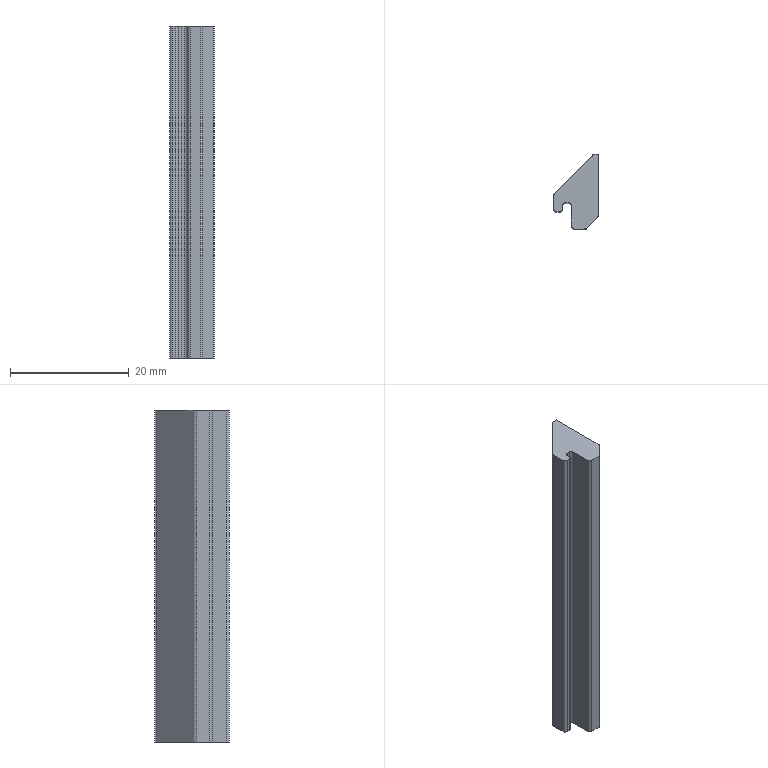Part | NX | features BREP 2 | 2 solids | 42 faces | box 7.556 x 12.583 x 56 mm | volume 6581 mm3 | plane 24 | cylinder 18 | commonest cylinder face diameters 1 x18
STEP:
#1=CARTESIAN_POINT('',(3.778,-3.929,-4.));
#2=VERTEX_POINT('',#1);
#3=CARTESIAN_POINT('',(3.778,-3.929,52.));
#4=VERTEX_POINT('',#3);
#5=CARTESIAN_POINT('',(3.778,-3.929,0.));
#6=DIRECTION('',(0.,0.,1.));
#7=VECTOR('',#6,1000.);
#8=LINE('',#5,#7);
#9=EDGE_CURVE('',#2,#4,#8,.T.);
#10=ORIENTED_EDGE('',*,*,#9,.T.);
#11=CARTESIAN_POINT('',(3.632,-4.282,52.));
#12=VERTEX_POINT('',#11);
#13=CARTESIAN_POINT('',(3.278,-3.929,52.));
#14=DIRECTION('',(0.,0.,1.));
#15=DIRECTION('',(1.,0.,0.));
#16=AXIS2_PLACEMENT_3D('',#13,#14,#15);
#17=CIRCLE('',#16,0.5);
#18=EDGE_CURVE('',#12,#4,#17,.T.);
#19=ORIENTED_EDGE('',*,*,#18,.F.);
#20=CARTESIAN_POINT('',(3.632,-4.282,-4.));
#21=VERTEX_POINT('',#20);
#22=CARTESIAN_POINT('',(3.632,-4.282,0.));
#23=DIRECTION('',(0.,0.,1.));
#24=VECTOR('',#23,1000.);
#25=LINE('',#22,#24);
#26=EDGE_CURVE('',#21,#12,#25,.T.);
#27=ORIENTED_EDGE('',*,*,#26,.F.);
#28=CARTESIAN_POINT('',(3.278,-3.929,-4.));
#29=DIRECTION('',(0.,0.,1.));
#30=DIRECTION('',(1.,0.,0.));
#31=AXIS2_PLACEMENT_3D('',#28,#29,#30);
#32=CIRCLE('',#31,0.5);
#33=EDGE_CURVE('',#21,#2,#32,.T.);
#34=ORIENTED_EDGE('',*,*,#33,.T.);
#35=EDGE_LOOP('',(#10,#19,#27,#34));
#36=FACE_BOUND('',#35,.T.);
#37=CARTESIAN_POINT('',(3.278,-3.929,0.));
#38=DIRECTION('',(0.,0.,1.));
#39=DIRECTION('',(-1.,0.,0.));
#40=AXIS2_PLACEMENT_3D('',#37,#38,#39);
#41=CYLINDRICAL_SURFACE('',#40,0.5);
#42=ADVANCED_FACE('',(#36),#41,.T.);
#43=ORIENTED_EDGE('',*,*,#26,.T.);
#44=CARTESIAN_POINT('',(1.768,-6.145,52.));
#45=VERTEX_POINT('',#44);
#46=CARTESIAN_POINT('',(3.632,-4.282,52.));
#47=DIRECTION('',(0.7071,0.7071,0.));
#48=VECTOR('',#47,1000.);
#49=LINE('',#46,#48);
#50=EDGE_CURVE('',#45,#12,#49,.T.);
#51=ORIENTED_EDGE('',*,*,#50,.F.);
#52=CARTESIAN_POINT('',(1.768,-6.145,-4.));
#53=VERTEX_POINT('',#52);
#54=CARTESIAN_POINT('',(1.768,-6.145,0.));
#55=DIRECTION('',(0.,0.,1.));
#56=VECTOR('',#55,1000.);
#57=LINE('',#54,#56);
#58=EDGE_CURVE('',#53,#45,#57,.T.);
#59=ORIENTED_EDGE('',*,*,#58,.F.);
#60=CARTESIAN_POINT('',(3.632,-4.282,-4.));
#61=DIRECTION('',(0.7071,0.7071,0.));
#62=VECTOR('',#61,1000.);
#63=LINE('',#60,#62);
#64=EDGE_CURVE('',#53,#21,#63,.T.);
#65=ORIENTED_EDGE('',*,*,#64,.T.);
#66=EDGE_LOOP('',(#43,#51,#59,#65));
#67=FACE_BOUND('',#66,.T.);
#68=CARTESIAN_POINT('',(3.632,-4.282,0.));
#69=DIRECTION('',(-0.7071,0.7071,0.));
#70=DIRECTION('',(0.7071,0.7071,0.));
#71=AXIS2_PLACEMENT_3D('',#68,#69,#70);
#72=PLANE('',#71);
#73=ADVANCED_FACE('',(#67),#72,.F.);
#74=ORIENTED_EDGE('',*,*,#58,.T.);
#75=CARTESIAN_POINT('',(1.415,-6.292,52.));
#76=VERTEX_POINT('',#75);
#77=CARTESIAN_POINT('',(1.415,-5.792,52.));
#78=DIRECTION('',(0.,0.,1.));
#79=DIRECTION('',(1.,0.,0.));
#80=AXIS2_PLACEMENT_3D('',#77,#78,#79);
#81=CIRCLE('',#80,0.5);
#82=EDGE_CURVE('',#76,#45,#81,.T.);
#83=ORIENTED_EDGE('',*,*,#82,.F.);
#84=CARTESIAN_POINT('',(1.415,-6.292,-4.));
#85=VERTEX_POINT('',#84);
#86=CARTESIAN_POINT('',(1.415,-6.292,0.));
#87=DIRECTION('',(0.,0.,1.));
#88=VECTOR('',#87,1000.);
#89=LINE('',#86,#88);
#90=EDGE_CURVE('',#85,#76,#89,.T.);
#91=ORIENTED_EDGE('',*,*,#90,.F.);
#92=CARTESIAN_POINT('',(1.415,-5.792,-4.));
#93=DIRECTION('',(0.,0.,1.));
#94=DIRECTION('',(1.,0.,0.));
#95=AXIS2_PLACEMENT_3D('',#92,#93,#94);
#96=CIRCLE('',#95,0.5);
#97=EDGE_CURVE('',#85,#53,#96,.T.);
#98=ORIENTED_EDGE('',*,*,#97,.T.);
#99=EDGE_LOOP('',(#74,#83,#91,#98));
#100=FACE_BOUND('',#99,.T.);
#101=CARTESIAN_POINT('',(1.415,-5.792,0.));
#102=DIRECTION('',(0.,0.,1.));
#103=DIRECTION('',(-1.,0.,0.));
#104=AXIS2_PLACEMENT_3D('',#101,#102,#103);
#105=CYLINDRICAL_SURFACE('',#104,0.5);
#106=ADVANCED_FACE('',(#100),#105,.T.);
#107=ORIENTED_EDGE('',*,*,#90,.T.);
#108=CARTESIAN_POINT('',(-0.278,-6.292,52.));
#109=VERTEX_POINT('',#108);
#110=CARTESIAN_POINT('',(-3.752,-6.292,52.));
#111=DIRECTION('',(1.,0.,0.));
#112=VECTOR('',#111,1000.);
#113=LINE('',#110,#112);
#114=EDGE_CURVE('',#109,#76,#113,.T.);
#115=ORIENTED_EDGE('',*,*,#114,.F.);
#116=CARTESIAN_POINT('',(-0.278,-6.292,-4.));
#117=VERTEX_POINT('',#116);
#118=CARTESIAN_POINT('',(-0.278,-6.292,0.));
#119=DIRECTION('',(0.,0.,1.));
#120=VECTOR('',#119,1000.);
#121=LINE('',#118,#120);
#122=EDGE_CURVE('',#117,#109,#121,.T.);
#123=ORIENTED_EDGE('',*,*,#122,.F.);
#124=CARTESIAN_POINT('',(-3.752,-6.292,-4.));
#125=DIRECTION('',(1.,0.,0.));
#126=VECTOR('',#125,1000.);
#127=LINE('',#124,#126);
#128=EDGE_CURVE('',#117,#85,#127,.T.);
#129=ORIENTED_EDGE('',*,*,#128,.T.);
#130=EDGE_LOOP('',(#107,#115,#123,#129));
#131=FACE_BOUND('',#130,.T.);
#132=CARTESIAN_POINT('',(1.415,-6.292,0.));
#133=DIRECTION('',(0.,1.,0.));
#134=DIRECTION('',(1.,0.,0.));
#135=AXIS2_PLACEMENT_3D('',#132,#133,#134);
#136=PLANE('',#135);
#137=ADVANCED_FACE('',(#131),#136,.F.);
#138=ORIENTED_EDGE('',*,*,#122,.T.);
#139=CARTESIAN_POINT('',(-0.778,-5.792,52.));
#140=VERTEX_POINT('',#139);
#141=CARTESIAN_POINT('',(-0.278,-5.792,52.));
#142=DIRECTION('',(0.,0.,1.));
#143=DIRECTION('',(1.,0.,0.));
#144=AXIS2_PLACEMENT_3D('',#141,#142,#143);
#145=CIRCLE('',#144,0.5);
#146=EDGE_CURVE('',#140,#109,#145,.T.);
#147=ORIENTED_EDGE('',*,*,#146,.F.);
#148=CARTESIAN_POINT('',(-0.778,-5.792,-4.));
#149=VERTEX_POINT('',#148);
#150=CARTESIAN_POINT('',(-0.778,-5.792,0.));
#151=DIRECTION('',(0.,0.,1.));
#152=VECTOR('',#151,1000.);
#153=LINE('',#150,#152);
#154=EDGE_CURVE('',#149,#140,#153,.T.);
#155=ORIENTED_EDGE('',*,*,#154,.F.);
#156=CARTESIAN_POINT('',(-0.278,-5.792,-4.));
#157=DIRECTION('',(0.,0.,1.));
#158=DIRECTION('',(1.,0.,0.));
#159=AXIS2_PLACEMENT_3D('',#156,#157,#158);
#160=CIRCLE('',#159,0.5);
#161=EDGE_CURVE('',#149,#117,#160,.T.);
#162=ORIENTED_EDGE('',*,*,#161,.T.);
#163=EDGE_LOOP('',(#138,#147,#155,#162));
#164=FACE_BOUND('',#163,.T.);
#165=CARTESIAN_POINT('',(-0.278,-5.792,0.));
#166=DIRECTION('',(0.,0.,1.));
#167=DIRECTION('',(-1.,0.,0.));
#168=AXIS2_PLACEMENT_3D('',#165,#166,#167);
#169=CYLINDRICAL_SURFACE('',#168,0.5);
#170=ADVANCED_FACE('',(#164),#169,.T.);
#171=ORIENTED_EDGE('',*,*,#154,.T.);
#172=CARTESIAN_POINT('',(-0.778,-2.392,52.));
#173=VERTEX_POINT('',#172);
#174=CARTESIAN_POINT('',(-0.778,-5.414,52.));
#175=DIRECTION('',(0.,-1.,0.));
#176=VECTOR('',#175,1000.);
#177=LINE('',#174,#176);
#178=EDGE_CURVE('',#173,#140,#177,.T.);
#179=ORIENTED_EDGE('',*,*,#178,.F.);
#180=CARTESIAN_POINT('',(-0.778,-2.392,-4.));
#181=VERTEX_POINT('',#180);
#182=CARTESIAN_POINT('',(-0.778,-2.392,0.));
#183=DIRECTION('',(0.,0.,1.));
#184=VECTOR('',#183,1000.);
#185=LINE('',#182,#184);
#186=EDGE_CURVE('',#181,#173,#185,.T.);
#187=ORIENTED_EDGE('',*,*,#186,.F.);
#188=CARTESIAN_POINT('',(-0.778,-5.414,-4.));
#189=DIRECTION('',(0.,-1.,0.));
#190=VECTOR('',#189,1000.);
#191=LINE('',#188,#190);
#192=EDGE_CURVE('',#181,#149,#191,.T.);
#193=ORIENTED_EDGE('',*,*,#192,.T.);
#194=EDGE_LOOP('',(#171,#179,#187,#193));
#195=FACE_BOUND('',#194,.T.);
#196=CARTESIAN_POINT('',(-0.778,-5.792,0.));
#197=DIRECTION('',(1.,0.,0.));
#198=DIRECTION('',(0.,-1.,0.));
#199=AXIS2_PLACEMENT_3D('',#196,#197,#198);
#200=PLANE('',#199);
#201=ADVANCED_FACE('',(#195),#200,.F.);
#202=ORIENTED_EDGE('',*,*,#186,.T.);
#203=CARTESIAN_POINT('',(-1.278,-1.892,52.));
#204=VERTEX_POINT('',#203);
#205=CARTESIAN_POINT('',(-1.278,-2.392,52.));
#206=DIRECTION('',(0.,0.,-1.));
#207=DIRECTION('',(1.,0.,0.));
#208=AXIS2_PLACEMENT_3D('',#205,#206,#207);
#209=CIRCLE('',#208,0.5);
#210=EDGE_CURVE('',#204,#173,#209,.T.);
#211=ORIENTED_EDGE('',*,*,#210,.F.);
#212=CARTESIAN_POINT('',(-1.278,-1.892,-4.));
#213=VERTEX_POINT('',#212);
#214=CARTESIAN_POINT('',(-1.278,-1.892,0.));
#215=DIRECTION('',(0.,0.,1.));
#216=VECTOR('',#215,1000.);
#217=LINE('',#214,#216);
#218=EDGE_CURVE('',#213,#204,#217,.T.);
#219=ORIENTED_EDGE('',*,*,#218,.F.);
#220=CARTESIAN_POINT('',(-1.278,-2.392,-4.));
#221=DIRECTION('',(0.,0.,-1.));
#222=DIRECTION('',(1.,0.,0.));
#223=AXIS2_PLACEMENT_3D('',#220,#221,#222);
#224=CIRCLE('',#223,0.5);
#225=EDGE_CURVE('',#213,#181,#224,.T.);
#226=ORIENTED_EDGE('',*,*,#225,.T.);
#227=EDGE_LOOP('',(#202,#211,#219,#226));
#228=FACE_BOUND('',#227,.T.);
#229=CARTESIAN_POINT('',(-1.278,-2.392,0.));
#230=DIRECTION('',(0.,0.,1.));
#231=DIRECTION('',(-1.,0.,0.));
#232=AXIS2_PLACEMENT_3D('',#229,#230,#231);
#233=CYLINDRICAL_SURFACE('',#232,0.5);
#234=ADVANCED_FACE('',(#228),#233,.F.);
#235=ORIENTED_EDGE('',*,*,#218,.T.);
#236=CARTESIAN_POINT('',(-1.778,-1.892,52.));
#237=VERTEX_POINT('',#236);
#238=CARTESIAN_POINT('',(-3.752,-1.892,52.));
#239=DIRECTION('',(1.,0.,0.));
#240=VECTOR('',#239,1000.);
#241=LINE('',#238,#240);
#242=EDGE_CURVE('',#237,#204,#241,.T.);
#243=ORIENTED_EDGE('',*,*,#242,.F.);
#244=CARTESIAN_POINT('',(-1.778,-1.892,-4.));
#245=VERTEX_POINT('',#244);
#246=CARTESIAN_POINT('',(-1.778,-1.892,0.));
#247=DIRECTION('',(0.,0.,1.));
#248=VECTOR('',#247,1000.);
#249=LINE('',#246,#248);
#250=EDGE_CURVE('',#245,#237,#249,.T.);
#251=ORIENTED_EDGE('',*,*,#250,.F.);
#252=CARTESIAN_POINT('',(-3.752,-1.892,-4.));
#253=DIRECTION('',(1.,0.,0.));
#254=VECTOR('',#253,1000.);
#255=LINE('',#252,#254);
#256=EDGE_CURVE('',#245,#213,#255,.T.);
#257=ORIENTED_EDGE('',*,*,#256,.T.);
#258=EDGE_LOOP('',(#235,#243,#251,#257));
#259=FACE_BOUND('',#258,.T.);
#260=CARTESIAN_POINT('',(-1.278,-1.892,0.));
#261=DIRECTION('',(0.,1.,0.));
#262=DIRECTION('',(1.,0.,0.));
#263=AXIS2_PLACEMENT_3D('',#260,#261,#262);
#264=PLANE('',#263);
#265=ADVANCED_FACE('',(#259),#264,.F.);
#266=ORIENTED_EDGE('',*,*,#250,.T.);
#267=CARTESIAN_POINT('',(-2.278,-2.392,52.));
#268=VERTEX_POINT('',#267);
#269=CARTESIAN_POINT('',(-1.778,-2.392,52.));
#270=DIRECTION('',(0.,0.,-1.));
#271=DIRECTION('',(1.,0.,0.));
#272=AXIS2_PLACEMENT_3D('',#269,#270,#271);
#273=CIRCLE('',#272,0.5);
#274=EDGE_CURVE('',#268,#237,#273,.T.);
#275=ORIENTED_EDGE('',*,*,#274,.F.);
#276=CARTESIAN_POINT('',(-2.278,-2.392,-4.));
#277=VERTEX_POINT('',#276);
#278=CARTESIAN_POINT('',(-2.278,-2.392,0.));
#279=DIRECTION('',(0.,0.,1.));
#280=VECTOR('',#279,1000.);
#281=LINE('',#278,#280);
#282=EDGE_CURVE('',#277,#268,#281,.T.);
#283=ORIENTED_EDGE('',*,*,#282,.F.);
#284=CARTESIAN_POINT('',(-1.778,-2.392,-4.));
#285=DIRECTION('',(0.,0.,-1.));
#286=DIRECTION('',(1.,0.,0.));
#287=AXIS2_PLACEMENT_3D('',#284,#285,#286);
#288=CIRCLE('',#287,0.5);
#289=EDGE_CURVE('',#277,#245,#288,.T.);
#290=ORIENTED_EDGE('',*,*,#289,.T.);
#291=EDGE_LOOP('',(#266,#275,#283,#290));
#292=FACE_BOUND('',#291,.T.);
#293=CARTESIAN_POINT('',(-1.778,-2.392,0.));
#294=DIRECTION('',(0.,0.,1.));
#295=DIRECTION('',(-1.,0.,0.));
#296=AXIS2_PLACEMENT_3D('',#293,#294,#295);
#297=CYLINDRICAL_SURFACE('',#296,0.5);
#298=ADVANCED_FACE('',(#292),#297,.F.);
#299=ORIENTED_EDGE('',*,*,#282,.T.);
#300=CARTESIAN_POINT('',(-2.278,-2.892,52.));
#301=VERTEX_POINT('',#300);
#302=CARTESIAN_POINT('',(-2.278,-5.414,52.));
#303=DIRECTION('',(0.,1.,0.));
#304=VECTOR('',#303,1000.);
#305=LINE('',#302,#304);
#306=EDGE_CURVE('',#301,#268,#305,.T.);
#307=ORIENTED_EDGE('',*,*,#306,.F.);
#308=CARTESIAN_POINT('',(-2.278,-2.892,-4.));
#309=VERTEX_POINT('',#308);
#310=CARTESIAN_POINT('',(-2.278,-2.892,0.));
#311=DIRECTION('',(0.,0.,1.));
#312=VECTOR('',#311,1000.);
#313=LINE('',#310,#312);
#314=EDGE_CURVE('',#309,#301,#313,.T.);
#315=ORIENTED_EDGE('',*,*,#314,.F.);
#316=CARTESIAN_POINT('',(-2.278,-5.414,-4.));
#317=DIRECTION('',(0.,1.,0.));
#318=VECTOR('',#317,1000.);
#319=LINE('',#316,#318);
#320=EDGE_CURVE('',#309,#277,#319,.T.);
#321=ORIENTED_EDGE('',*,*,#320,.T.);
#322=EDGE_LOOP('',(#299,#307,#315,#321));
#323=FACE_BOUND('',#322,.T.);
#324=CARTESIAN_POINT('',(-2.278,-2.392,0.));
#325=DIRECTION('',(-1.,0.,0.));
#326=DIRECTION('',(0.,1.,0.));
#327=AXIS2_PLACEMENT_3D('',#324,#325,#326);
#328=PLANE('',#327);
#329=ADVANCED_FACE('',(#323),#328,.F.);
#330=ORIENTED_EDGE('',*,*,#314,.T.);
#331=CARTESIAN_POINT('',(-2.778,-3.392,52.));
#332=VERTEX_POINT('',#331);
#333=CARTESIAN_POINT('',(-2.778,-2.892,52.));
#334=DIRECTION('',(0.,0.,1.));
#335=DIRECTION('',(1.,0.,0.));
#336=AXIS2_PLACEMENT_3D('',#333,#334,#335);
#337=CIRCLE('',#336,0.5);
#338=EDGE_CURVE('',#332,#301,#337,.T.);
#339=ORIENTED_EDGE('',*,*,#338,.F.);
#340=CARTESIAN_POINT('',(-2.778,-3.392,-4.));
#341=VERTEX_POINT('',#340);
#342=CARTESIAN_POINT('',(-2.778,-3.392,0.));
#343=DIRECTION('',(0.,0.,1.));
#344=VECTOR('',#343,1000.);
#345=LINE('',#342,#344);
#346=EDGE_CURVE('',#341,#332,#345,.T.);
#347=ORIENTED_EDGE('',*,*,#346,.F.);
#348=CARTESIAN_POINT('',(-2.778,-2.892,-4.));
#349=DIRECTION('',(0.,0.,1.));
#350=DIRECTION('',(1.,0.,0.));
#351=AXIS2_PLACEMENT_3D('',#348,#349,#350);
#352=CIRCLE('',#351,0.5);
#353=EDGE_CURVE('',#341,#309,#352,.T.);
#354=ORIENTED_EDGE('',*,*,#353,.T.);
#355=EDGE_LOOP('',(#330,#339,#347,#354));
#356=FACE_BOUND('',#355,.T.);
#357=CARTESIAN_POINT('',(-2.778,-2.892,0.));
#358=DIRECTION('',(0.,0.,1.));
#359=DIRECTION('',(-1.,0.,0.));
#360=AXIS2_PLACEMENT_3D('',#357,#358,#359);
#361=CYLINDRICAL_SURFACE('',#360,0.5);
#362=ADVANCED_FACE('',(#356),#361,.T.);
#363=ORIENTED_EDGE('',*,*,#346,.T.);
#364=CARTESIAN_POINT('',(-3.278,-3.392,52.));
#365=VERTEX_POINT('',#364);
#366=CARTESIAN_POINT('',(-3.752,-3.392,52.));
#367=DIRECTION('',(1.,0.,0.));
#368=VECTOR('',#367,1000.);
#369=LINE('',#366,#368);
#370=EDGE_CURVE('',#365,#332,#369,.T.);
#371=ORIENTED_EDGE('',*,*,#370,.F.);
#372=CARTESIAN_POINT('',(-3.278,-3.392,-4.));
#373=VERTEX_POINT('',#372);
#374=CARTESIAN_POINT('',(-3.278,-3.392,0.));
#375=DIRECTION('',(0.,0.,1.));
#376=VECTOR('',#375,1000.);
#377=LINE('',#374,#376);
#378=EDGE_CURVE('',#373,#365,#377,.T.);
#379=ORIENTED_EDGE('',*,*,#378,.F.);
#380=CARTESIAN_POINT('',(-3.752,-3.392,-4.));
#381=DIRECTION('',(1.,0.,0.));
#382=VECTOR('',#381,1000.);
#383=LINE('',#380,#382);
#384=EDGE_CURVE('',#373,#341,#383,.T.);
#385=ORIENTED_EDGE('',*,*,#384,.T.);
#386=EDGE_LOOP('',(#363,#371,#379,#385));
#387=FACE_BOUND('',#386,.T.);
#388=CARTESIAN_POINT('',(-2.778,-3.392,0.));
#389=DIRECTION('',(0.,1.,0.));
#390=DIRECTION('',(1.,0.,0.));
#391=AXIS2_PLACEMENT_3D('',#388,#389,#390);
#392=PLANE('',#391);
#393=ADVANCED_FACE('',(#387),#392,.F.);
#394=ORIENTED_EDGE('',*,*,#378,.T.);
#395=CARTESIAN_POINT('',(-3.778,-2.892,52.));
#396=VERTEX_POINT('',#395);
#397=CARTESIAN_POINT('',(-3.278,-2.892,52.));
#398=DIRECTION('',(0.,0.,1.));
#399=DIRECTION('',(1.,0.,0.));
#400=AXIS2_PLACEMENT_3D('',#397,#398,#399);
#401=CIRCLE('',#400,0.5);
#402=EDGE_CURVE('',#396,#365,#401,.T.);
#403=ORIENTED_EDGE('',*,*,#402,.F.);
#404=CARTESIAN_POINT('',(-3.778,-2.892,-4.));
#405=VERTEX_POINT('',#404);
#406=CARTESIAN_POINT('',(-3.778,-2.892,0.));
#407=DIRECTION('',(0.,0.,1.));
#408=VECTOR('',#407,1000.);
#409=LINE('',#406,#408);
#410=EDGE_CURVE('',#405,#396,#409,.T.);
#411=ORIENTED_EDGE('',*,*,#410,.F.);
#412=CARTESIAN_POINT('',(-3.278,-2.892,-4.));
#413=DIRECTION('',(0.,0.,1.));
#414=DIRECTION('',(1.,0.,0.));
#415=AXIS2_PLACEMENT_3D('',#412,#413,#414);
#416=CIRCLE('',#415,0.5);
#417=EDGE_CURVE('',#405,#373,#416,.T.);
#418=ORIENTED_EDGE('',*,*,#417,.T.);
#419=EDGE_LOOP('',(#394,#403,#411,#418));
#420=FACE_BOUND('',#419,.T.);
#421=CARTESIAN_POINT('',(-3.278,-2.892,0.));
#422=DIRECTION('',(0.,0.,1.));
#423=DIRECTION('',(-1.,0.,0.));
#424=AXIS2_PLACEMENT_3D('',#421,#422,#423);
#425=CYLINDRICAL_SURFACE('',#424,0.5);
#426=ADVANCED_FACE('',(#420),#425,.T.);
#427=ORIENTED_EDGE('',*,*,#410,.T.);
#428=CARTESIAN_POINT('',(-3.778,-0.6987,52.));
#429=VERTEX_POINT('',#428);
#430=CARTESIAN_POINT('',(-3.778,-5.414,52.));
#431=DIRECTION('',(0.,-1.,0.));
#432=VECTOR('',#431,1000.);
#433=LINE('',#430,#432);
#434=EDGE_CURVE('',#429,#396,#433,.T.);
#435=ORIENTED_EDGE('',*,*,#434,.F.);
#436=CARTESIAN_POINT('',(-3.778,-0.6987,-4.));
#437=VERTEX_POINT('',#436);
#438=CARTESIAN_POINT('',(-3.778,-0.6987,0.));
#439=DIRECTION('',(0.,0.,1.));
#440=VECTOR('',#439,1000.);
#441=LINE('',#438,#440);
#442=EDGE_CURVE('',#437,#429,#441,.T.);
#443=ORIENTED_EDGE('',*,*,#442,.F.);
#444=CARTESIAN_POINT('',(-3.778,-5.414,-4.));
#445=DIRECTION('',(0.,-1.,0.));
#446=VECTOR('',#445,1000.);
#447=LINE('',#444,#446);
#448=EDGE_CURVE('',#437,#405,#447,.T.);
#449=ORIENTED_EDGE('',*,*,#448,.T.);
#450=EDGE_LOOP('',(#427,#435,#443,#449));
#451=FACE_BOUND('',#450,.T.);
#452=CARTESIAN_POINT('',(-3.778,-2.892,0.));
#453=DIRECTION('',(1.,0.,0.));
#454=DIRECTION('',(0.,-1.,0.));
#455=AXIS2_PLACEMENT_3D('',#452,#453,#454);
#456=PLANE('',#455);
#457=ADVANCED_FACE('',(#451),#456,.F.);
#458=ORIENTED_EDGE('',*,*,#442,.T.);
#459=CARTESIAN_POINT('',(-3.632,-0.3452,52.));
#460=VERTEX_POINT('',#459);
#461=CARTESIAN_POINT('',(-3.278,-0.6987,52.));
#462=DIRECTION('',(0.,0.,1.));
#463=DIRECTION('',(1.,0.,0.));
#464=AXIS2_PLACEMENT_3D('',#461,#462,#463);
#465=CIRCLE('',#464,0.5);
#466=EDGE_CURVE('',#460,#429,#465,.T.);
#467=ORIENTED_EDGE('',*,*,#466,.F.);
#468=CARTESIAN_POINT('',(-3.632,-0.3452,-4.));
#469=VERTEX_POINT('',#468);
#470=CARTESIAN_POINT('',(-3.632,-0.3452,0.));
#471=DIRECTION('',(0.,0.,1.));
#472=VECTOR('',#471,1000.);
#473=LINE('',#470,#472);
#474=EDGE_CURVE('',#469,#460,#473,.T.);
#475=ORIENTED_EDGE('',*,*,#474,.F.);
#476=CARTESIAN_POINT('',(-3.278,-0.6987,-4.));
#477=DIRECTION('',(0.,0.,1.));
#478=DIRECTION('',(1.,0.,0.));
#479=AXIS2_PLACEMENT_3D('',#476,#477,#478);
#480=CIRCLE('',#479,0.5);
#481=EDGE_CURVE('',#469,#437,#480,.T.);
#482=ORIENTED_EDGE('',*,*,#481,.T.);
#483=EDGE_LOOP('',(#458,#467,#475,#482));
#484=FACE_BOUND('',#483,.T.);
#485=CARTESIAN_POINT('',(-3.278,-0.6987,0.));
#486=DIRECTION('',(0.,0.,1.));
#487=DIRECTION('',(-1.,0.,0.));
#488=AXIS2_PLACEMENT_3D('',#485,#486,#487);
#489=CYLINDRICAL_SURFACE('',#488,0.5);
#490=ADVANCED_FACE('',(#484),#489,.T.);
#491=ORIENTED_EDGE('',*,*,#474,.T.);
#492=CARTESIAN_POINT('',(2.652,5.938,52.));
#493=VERTEX_POINT('',#492);
#494=CARTESIAN_POINT('',(-3.632,-0.3452,52.));
#495=DIRECTION('',(-0.7071,-0.7071,0.));
#496=VECTOR('',#495,1000.);
#497=LINE('',#494,#496);
#498=EDGE_CURVE('',#493,#460,#497,.T.);
#499=ORIENTED_EDGE('',*,*,#498,.F.);
#500=CARTESIAN_POINT('',(2.652,5.938,-4.));
#501=VERTEX_POINT('',#500);
#502=CARTESIAN_POINT('',(2.652,5.938,0.));
#503=DIRECTION('',(0.,0.,1.));
#504=VECTOR('',#503,1000.);
#505=LINE('',#502,#504);
#506=EDGE_CURVE('',#501,#493,#505,.T.);
#507=ORIENTED_EDGE('',*,*,#506,.F.);
#508=CARTESIAN_POINT('',(-3.632,-0.3452,-4.));
#509=DIRECTION('',(-0.7071,-0.7071,0.));
#510=VECTOR('',#509,1000.);
#511=LINE('',#508,#510);
#512=EDGE_CURVE('',#501,#469,#511,.T.);
#513=ORIENTED_EDGE('',*,*,#512,.T.);
#514=EDGE_LOOP('',(#491,#499,#507,#513));
#515=FACE_BOUND('',#514,.T.);
#516=CARTESIAN_POINT('',(-3.632,-0.3452,0.));
#517=DIRECTION('',(0.7071,-0.7071,0.));
#518=DIRECTION('',(-0.7071,-0.7071,0.));
#519=AXIS2_PLACEMENT_3D('',#516,#517,#518);
#520=PLANE('',#519);
#521=ADVANCED_FACE('',(#515),#520,.F.);
#522=ORIENTED_EDGE('',*,*,#506,.T.);
#523=CARTESIAN_POINT('',(2.798,6.292,52.));
#524=VERTEX_POINT('',#523);
#525=CARTESIAN_POINT('',(2.298,6.292,52.));
#526=DIRECTION('',(0.,0.,-1.));
#527=DIRECTION('',(1.,0.,0.));
#528=AXIS2_PLACEMENT_3D('',#525,#526,#527);
#529=CIRCLE('',#528,0.5);
#530=EDGE_CURVE('',#524,#493,#529,.T.);
#531=ORIENTED_EDGE('',*,*,#530,.F.);
#532=CARTESIAN_POINT('',(2.798,6.292,-4.));
#533=VERTEX_POINT('',#532);
#534=CARTESIAN_POINT('',(2.798,6.292,0.));
#535=DIRECTION('',(0.,0.,1.));
#536=VECTOR('',#535,1000.);
#537=LINE('',#534,#536);
#538=EDGE_CURVE('',#533,#524,#537,.T.);
#539=ORIENTED_EDGE('',*,*,#538,.F.);
#540=CARTESIAN_POINT('',(2.298,6.292,-4.));
#541=DIRECTION('',(0.,0.,-1.));
#542=DIRECTION('',(1.,0.,0.));
#543=AXIS2_PLACEMENT_3D('',#540,#541,#542);
#544=CIRCLE('',#543,0.5);
#545=EDGE_CURVE('',#533,#501,#544,.T.);
#546=ORIENTED_EDGE('',*,*,#545,.T.);
#547=EDGE_LOOP('',(#522,#531,#539,#546));
#548=FACE_BOUND('',#547,.T.);
#549=CARTESIAN_POINT('',(2.298,6.292,0.));
#550=DIRECTION('',(0.,0.,1.));
#551=DIRECTION('',(-1.,0.,0.));
#552=AXIS2_PLACEMENT_3D('',#549,#550,#551);
#553=CYLINDRICAL_SURFACE('',#552,0.5);
#554=ADVANCED_FACE('',(#548),#553,.F.);
#555=ORIENTED_EDGE('',*,*,#538,.T.);
#556=CARTESIAN_POINT('',(3.778,6.292,52.));
#557=VERTEX_POINT('',#556);
#558=CARTESIAN_POINT('',(-3.752,6.292,52.));
#559=DIRECTION('',(-1.,0.,0.));
#560=VECTOR('',#559,1000.);
#561=LINE('',#558,#560);
#562=EDGE_CURVE('',#557,#524,#561,.T.);
#563=ORIENTED_EDGE('',*,*,#562,.F.);
#564=CARTESIAN_POINT('',(3.778,6.292,-4.));
#565=VERTEX_POINT('',#564);
#566=CARTESIAN_POINT('',(3.778,6.292,0.));
#567=DIRECTION('',(0.,0.,1.));
#568=VECTOR('',#567,1000.);
#569=LINE('',#566,#568);
#570=EDGE_CURVE('',#565,#557,#569,.T.);
#571=ORIENTED_EDGE('',*,*,#570,.F.);
#572=CARTESIAN_POINT('',(-3.752,6.292,-4.));
#573=DIRECTION('',(-1.,0.,0.));
#574=VECTOR('',#573,1000.);
#575=LINE('',#572,#574);
#576=EDGE_CURVE('',#565,#533,#575,.T.);
#577=ORIENTED_EDGE('',*,*,#576,.T.);
#578=EDGE_LOOP('',(#555,#563,#571,#577));
#579=FACE_BOUND('',#578,.T.);
#580=CARTESIAN_POINT('',(-3.752,6.292,0.));
#581=DIRECTION('',(0.,-1.,0.));
#582=DIRECTION('',(-1.,0.,0.));
#583=AXIS2_PLACEMENT_3D('',#580,#581,#582);
#584=PLANE('',#583);
#585=ADVANCED_FACE('',(#579),#584,.F.);
#586=CARTESIAN_POINT('',(3.778,-5.414,-4.));
#587=DIRECTION('',(0.,1.,0.));
#588=VECTOR('',#587,1000.);
#589=LINE('',#586,#588);
#590=EDGE_CURVE('',#2,#565,#589,.T.);
#591=ORIENTED_EDGE('',*,*,#590,.T.);
#592=ORIENTED_EDGE('',*,*,#570,.T.);
#593=CARTESIAN_POINT('',(3.778,-5.414,52.));
#594=DIRECTION('',(0.,1.,0.));
#595=VECTOR('',#594,1000.);
#596=LINE('',#593,#595);
#597=EDGE_CURVE('',#4,#557,#596,.T.);
#598=ORIENTED_EDGE('',*,*,#597,.F.);
#599=ORIENTED_EDGE('',*,*,#9,.F.);
#600=EDGE_LOOP('',(#591,#592,#598,#599));
#601=FACE_BOUND('',#600,.T.);
#602=CARTESIAN_POINT('',(3.778,8.984,0.));
#603=DIRECTION('',(-1.,0.,0.));
#604=DIRECTION('',(0.,1.,0.));
#605=AXIS2_PLACEMENT_3D('',#602,#603,#604);
#606=PLANE('',#605);
#607=ADVANCED_FACE('',(#601),#606,.F.);
#608=ORIENTED_EDGE('',*,*,#562,.T.);
#609=ORIENTED_EDGE('',*,*,#530,.T.);
#610=ORIENTED_EDGE('',*,*,#498,.T.);
#611=ORIENTED_EDGE('',*,*,#466,.T.);
#612=ORIENTED_EDGE('',*,*,#434,.T.);
#613=ORIENTED_EDGE('',*,*,#402,.T.);
#614=ORIENTED_EDGE('',*,*,#370,.T.);
#615=ORIENTED_EDGE('',*,*,#338,.T.);
#616=ORIENTED_EDGE('',*,*,#306,.T.);
#617=ORIENTED_EDGE('',*,*,#274,.T.);
#618=ORIENTED_EDGE('',*,*,#242,.T.);
#619=ORIENTED_EDGE('',*,*,#210,.T.);
#620=ORIENTED_EDGE('',*,*,#178,.T.);
#621=ORIENTED_EDGE('',*,*,#146,.T.);
#622=ORIENTED_EDGE('',*,*,#114,.T.);
#623=ORIENTED_EDGE('',*,*,#82,.T.);
#624=ORIENTED_EDGE('',*,*,#50,.T.);
#625=ORIENTED_EDGE('',*,*,#18,.T.);
#626=ORIENTED_EDGE('',*,*,#597,.T.);
#627=EDGE_LOOP('',(#608,#609,#610,#611,#612,#613,#614,#615,#616,#617,#618,#619,#620,#621,#622,#623,#624,#625,#626));
#628=FACE_BOUND('',#627,.T.);
#629=CARTESIAN_POINT('',(-3.752,-5.414,52.));
#630=DIRECTION('',(0.,0.,1.));
#631=DIRECTION('',(-1.,0.,0.));
#632=AXIS2_PLACEMENT_3D('',#629,#630,#631);
#633=PLANE('',#632);
#634=ADVANCED_FACE('',(#628),#633,.T.);
#635=ORIENTED_EDGE('',*,*,#576,.F.);
#636=ORIENTED_EDGE('',*,*,#590,.F.);
#637=ORIENTED_EDGE('',*,*,#33,.F.);
#638=ORIENTED_EDGE('',*,*,#64,.F.);
#639=ORIENTED_EDGE('',*,*,#97,.F.);
#640=ORIENTED_EDGE('',*,*,#128,.F.);
#641=ORIENTED_EDGE('',*,*,#161,.F.);
#642=ORIENTED_EDGE('',*,*,#192,.F.);
#643=ORIENTED_EDGE('',*,*,#225,.F.);
#644=ORIENTED_EDGE('',*,*,#256,.F.);
#645=ORIENTED_EDGE('',*,*,#289,.F.);
#646=ORIENTED_EDGE('',*,*,#320,.F.);
#647=ORIENTED_EDGE('',*,*,#353,.F.);
#648=ORIENTED_EDGE('',*,*,#384,.F.);
#649=ORIENTED_EDGE('',*,*,#417,.F.);
#650=ORIENTED_EDGE('',*,*,#448,.F.);
#651=ORIENTED_EDGE('',*,*,#481,.F.);
#652=ORIENTED_EDGE('',*,*,#512,.F.);
#653=ORIENTED_EDGE('',*,*,#545,.F.);
#654=EDGE_LOOP('',(#635,#636,#637,#638,#639,#640,#641,#642,#643,#644,#645,#646,#647,#648,#649,#650,#651,#652,#653));
#655=FACE_BOUND('',#654,.T.);
#656=CARTESIAN_POINT('',(-3.752,-5.414,-4.));
#657=DIRECTION('',(0.,0.,1.));
#658=DIRECTION('',(-1.,0.,0.));
#659=AXIS2_PLACEMENT_3D('',#656,#657,#658);
#660=PLANE('',#659);
#661=ADVANCED_FACE('',(#655),#660,.F.);
#662=CLOSED_SHELL('',(#42,#73,#106,#137,#170,#201,#234,#265,#298,#329,#362,#393,#426,#457,#490,#521,#554,#585,#607,#634,#661));
#663=MANIFOLD_SOLID_BREP('',#662);
#664=CARTESIAN_POINT('',(3.778,-3.929,-4.));
#665=VERTEX_POINT('',#664);
#666=CARTESIAN_POINT('',(3.778,-3.929,52.));
#667=VERTEX_POINT('',#666);
#668=CARTESIAN_POINT('',(3.778,-3.929,0.));
#669=DIRECTION('',(0.,0.,1.));
#670=VECTOR('',#669,1000.);
#671=LINE('',#668,#670);
#672=EDGE_CURVE('',#665,#667,#671,.T.);
#673=ORIENTED_EDGE('',*,*,#672,.T.);
#674=CARTESIAN_POINT('',(3.632,-4.282,52.));
#675=VERTEX_POINT('',#674);
#676=CARTESIAN_POINT('',(3.278,-3.929,52.));
#677=DIRECTION('',(0.,0.,1.));
#678=DIRECTION('',(1.,0.,0.));
#679=AXIS2_PLACEMENT_3D('',#676,#677,#678);
#680=CIRCLE('',#679,0.5);
#681=EDGE_CURVE('',#675,#667,#680,.T.);
#682=ORIENTED_EDGE('',*,*,#681,.F.);
#683=CARTESIAN_POINT('',(3.632,-4.282,-4.));
#684=VERTEX_POINT('',#683);
#685=CARTESIAN_POINT('',(3.632,-4.282,0.));
#686=DIRECTION('',(0.,0.,1.));
#687=VECTOR('',#686,1000.);
#688=LINE('',#685,#687);
#689=EDGE_CURVE('',#684,#675,#688,.T.);
#690=ORIENTED_EDGE('',*,*,#689,.F.);
#691=CARTESIAN_POINT('',(3.278,-3.929,-4.));
#692=DIRECTION('',(0.,0.,1.));
#693=DIRECTION('',(1.,0.,0.));
#694=AXIS2_PLACEMENT_3D('',#691,#692,#693);
#695=CIRCLE('',#694,0.5);
#696=EDGE_CURVE('',#684,#665,#695,.T.);
#697=ORIENTED_EDGE('',*,*,#696,.T.);
#698=EDGE_LOOP('',(#673,#682,#690,#697));
#699=FACE_BOUND('',#698,.T.);
#700=CARTESIAN_POINT('',(3.278,-3.929,0.));
#701=DIRECTION('',(0.,0.,1.));
#702=DIRECTION('',(-1.,0.,0.));
#703=AXIS2_PLACEMENT_3D('',#700,#701,#702);
#704=CYLINDRICAL_SURFACE('',#703,0.5);
#705=ADVANCED_FACE('',(#699),#704,.T.);
#706=ORIENTED_EDGE('',*,*,#689,.T.);
#707=CARTESIAN_POINT('',(1.768,-6.145,52.));
#708=VERTEX_POINT('',#707);
#709=CARTESIAN_POINT('',(3.632,-4.282,52.));
#710=DIRECTION('',(0.7071,0.7071,0.));
#711=VECTOR('',#710,1000.);
#712=LINE('',#709,#711);
#713=EDGE_CURVE('',#708,#675,#712,.T.);
#714=ORIENTED_EDGE('',*,*,#713,.F.);
#715=CARTESIAN_POINT('',(1.768,-6.145,-4.));
#716=VERTEX_POINT('',#715);
#717=CARTESIAN_POINT('',(1.768,-6.145,0.));
#718=DIRECTION('',(0.,0.,1.));
#719=VECTOR('',#718,1000.);
#720=LINE('',#717,#719);
#721=EDGE_CURVE('',#716,#708,#720,.T.);
#722=ORIENTED_EDGE('',*,*,#721,.F.);
#723=CARTESIAN_POINT('',(3.632,-4.282,-4.));
#724=DIRECTION('',(0.7071,0.7071,0.));
#725=VECTOR('',#724,1000.);
#726=LINE('',#723,#725);
#727=EDGE_CURVE('',#716,#684,#726,.T.);
#728=ORIENTED_EDGE('',*,*,#727,.T.);
#729=EDGE_LOOP('',(#706,#714,#722,#728));
#730=FACE_BOUND('',#729,.T.);
#731=CARTESIAN_POINT('',(3.632,-4.282,0.));
#732=DIRECTION('',(-0.7071,0.7071,0.));
#733=DIRECTION('',(0.7071,0.7071,0.));
#734=AXIS2_PLACEMENT_3D('',#731,#732,#733);
#735=PLANE('',#734);
#736=ADVANCED_FACE('',(#730),#735,.F.);
#737=ORIENTED_EDGE('',*,*,#721,.T.);
#738=CARTESIAN_POINT('',(1.415,-6.292,52.));
#739=VERTEX_POINT('',#738);
#740=CARTESIAN_POINT('',(1.415,-5.792,52.));
#741=DIRECTION('',(0.,0.,1.));
#742=DIRECTION('',(1.,0.,0.));
#743=AXIS2_PLACEMENT_3D('',#740,#741,#742);
#744=CIRCLE('',#743,0.5);
#745=EDGE_CURVE('',#739,#708,#744,.T.);
#746=ORIENTED_EDGE('',*,*,#745,.F.);
#747=CARTESIAN_POINT('',(1.415,-6.292,-4.));
#748=VERTEX_POINT('',#747);
#749=CARTESIAN_POINT('',(1.415,-6.292,0.));
#750=DIRECTION('',(0.,0.,1.));
#751=VECTOR('',#750,1000.);
#752=LINE('',#749,#751);
#753=EDGE_CURVE('',#748,#739,#752,.T.);
#754=ORIENTED_EDGE('',*,*,#753,.F.);
#755=CARTESIAN_POINT('',(1.415,-5.792,-4.));
#756=DIRECTION('',(0.,0.,1.));
#757=DIRECTION('',(1.,0.,0.));
#758=AXIS2_PLACEMENT_3D('',#755,#756,#757);
#759=CIRCLE('',#758,0.5);
#760=EDGE_CURVE('',#748,#716,#759,.T.);
#761=ORIENTED_EDGE('',*,*,#760,.T.);
#762=EDGE_LOOP('',(#737,#746,#754,#761));
#763=FACE_BOUND('',#762,.T.);
#764=CARTESIAN_POINT('',(1.415,-5.792,0.));
#765=DIRECTION('',(0.,0.,1.));
#766=DIRECTION('',(-1.,0.,0.));
#767=AXIS2_PLACEMENT_3D('',#764,#765,#766);
#768=CYLINDRICAL_SURFACE('',#767,0.5);
#769=ADVANCED_FACE('',(#763),#768,.T.);
#770=ORIENTED_EDGE('',*,*,#753,.T.);
#771=CARTESIAN_POINT('',(-0.278,-6.292,52.));
#772=VERTEX_POINT('',#771);
#773=CARTESIAN_POINT('',(-3.752,-6.292,52.));
#774=DIRECTION('',(1.,0.,0.));
#775=VECTOR('',#774,1000.);
#776=LINE('',#773,#775);
#777=EDGE_CURVE('',#772,#739,#776,.T.);
#778=ORIENTED_EDGE('',*,*,#777,.F.);
#779=CARTESIAN_POINT('',(-0.278,-6.292,-4.));
#780=VERTEX_POINT('',#779);
#781=CARTESIAN_POINT('',(-0.278,-6.292,0.));
#782=DIRECTION('',(0.,0.,1.));
#783=VECTOR('',#782,1000.);
#784=LINE('',#781,#783);
#785=EDGE_CURVE('',#780,#772,#784,.T.);
#786=ORIENTED_EDGE('',*,*,#785,.F.);
#787=CARTESIAN_POINT('',(-3.752,-6.292,-4.));
#788=DIRECTION('',(1.,0.,0.));
#789=VECTOR('',#788,1000.);
#790=LINE('',#787,#789);
#791=EDGE_CURVE('',#780,#748,#790,.T.);
#792=ORIENTED_EDGE('',*,*,#791,.T.);
#793=EDGE_LOOP('',(#770,#778,#786,#792));
#794=FACE_BOUND('',#793,.T.);
#795=CARTESIAN_POINT('',(1.415,-6.292,0.));
#796=DIRECTION('',(0.,1.,0.));
#797=DIRECTION('',(1.,0.,0.));
#798=AXIS2_PLACEMENT_3D('',#795,#796,#797);
#799=PLANE('',#798);
#800=ADVANCED_FACE('',(#794),#799,.F.);
#801=ORIENTED_EDGE('',*,*,#785,.T.);
#802=CARTESIAN_POINT('',(-0.778,-5.792,52.));
#803=VERTEX_POINT('',#802);
#804=CARTESIAN_POINT('',(-0.278,-5.792,52.));
#805=DIRECTION('',(0.,0.,1.));
#806=DIRECTION('',(1.,0.,0.));
#807=AXIS2_PLACEMENT_3D('',#804,#805,#806);
#808=CIRCLE('',#807,0.5);
#809=EDGE_CURVE('',#803,#772,#808,.T.);
#810=ORIENTED_EDGE('',*,*,#809,.F.);
#811=CARTESIAN_POINT('',(-0.778,-5.792,-4.));
#812=VERTEX_POINT('',#811);
#813=CARTESIAN_POINT('',(-0.778,-5.792,0.));
#814=DIRECTION('',(0.,0.,1.));
#815=VECTOR('',#814,1000.);
#816=LINE('',#813,#815);
#817=EDGE_CURVE('',#812,#803,#816,.T.);
#818=ORIENTED_EDGE('',*,*,#817,.F.);
#819=CARTESIAN_POINT('',(-0.278,-5.792,-4.));
#820=DIRECTION('',(0.,0.,1.));
#821=DIRECTION('',(1.,0.,0.));
#822=AXIS2_PLACEMENT_3D('',#819,#820,#821);
#823=CIRCLE('',#822,0.5);
#824=EDGE_CURVE('',#812,#780,#823,.T.);
#825=ORIENTED_EDGE('',*,*,#824,.T.);
#826=EDGE_LOOP('',(#801,#810,#818,#825));
#827=FACE_BOUND('',#826,.T.);
#828=CARTESIAN_POINT('',(-0.278,-5.792,0.));
#829=DIRECTION('',(0.,0.,1.));
#830=DIRECTION('',(-1.,0.,0.));
#831=AXIS2_PLACEMENT_3D('',#828,#829,#830);
#832=CYLINDRICAL_SURFACE('',#831,0.5);
#833=ADVANCED_FACE('',(#827),#832,.T.);
#834=ORIENTED_EDGE('',*,*,#817,.T.);
#835=CARTESIAN_POINT('',(-0.778,-2.392,52.));
#836=VERTEX_POINT('',#835);
#837=CARTESIAN_POINT('',(-0.778,-5.414,52.));
#838=DIRECTION('',(0.,-1.,0.));
#839=VECTOR('',#838,1000.);
#840=LINE('',#837,#839);
#841=EDGE_CURVE('',#836,#803,#840,.T.);
#842=ORIENTED_EDGE('',*,*,#841,.F.);
#843=CARTESIAN_POINT('',(-0.778,-2.392,-4.));
#844=VERTEX_POINT('',#843);
#845=CARTESIAN_POINT('',(-0.778,-2.392,0.));
#846=DIRECTION('',(0.,0.,1.));
#847=VECTOR('',#846,1000.);
#848=LINE('',#845,#847);
#849=EDGE_CURVE('',#844,#836,#848,.T.);
#850=ORIENTED_EDGE('',*,*,#849,.F.);
#851=CARTESIAN_POINT('',(-0.778,-5.414,-4.));
#852=DIRECTION('',(0.,-1.,0.));
#853=VECTOR('',#852,1000.);
#854=LINE('',#851,#853);
#855=EDGE_CURVE('',#844,#812,#854,.T.);
#856=ORIENTED_EDGE('',*,*,#855,.T.);
#857=EDGE_LOOP('',(#834,#842,#850,#856));
#858=FACE_BOUND('',#857,.T.);
#859=CARTESIAN_POINT('',(-0.778,-5.792,0.));
#860=DIRECTION('',(1.,0.,0.));
#861=DIRECTION('',(0.,-1.,0.));
#862=AXIS2_PLACEMENT_3D('',#859,#860,#861);
#863=PLANE('',#862);
#864=ADVANCED_FACE('',(#858),#863,.F.);
#865=ORIENTED_EDGE('',*,*,#849,.T.);
#866=CARTESIAN_POINT('',(-1.278,-1.892,52.));
#867=VERTEX_POINT('',#866);
#868=CARTESIAN_POINT('',(-1.278,-2.392,52.));
#869=DIRECTION('',(0.,0.,-1.));
#870=DIRECTION('',(1.,0.,0.));
#871=AXIS2_PLACEMENT_3D('',#868,#869,#870);
#872=CIRCLE('',#871,0.5);
#873=EDGE_CURVE('',#867,#836,#872,.T.);
#874=ORIENTED_EDGE('',*,*,#873,.F.);
#875=CARTESIAN_POINT('',(-1.278,-1.892,-4.));
#876=VERTEX_POINT('',#875);
#877=CARTESIAN_POINT('',(-1.278,-1.892,0.));
#878=DIRECTION('',(0.,0.,1.));
#879=VECTOR('',#878,1000.);
#880=LINE('',#877,#879);
#881=EDGE_CURVE('',#876,#867,#880,.T.);
#882=ORIENTED_EDGE('',*,*,#881,.F.);
#883=CARTESIAN_POINT('',(-1.278,-2.392,-4.));
#884=DIRECTION('',(0.,0.,-1.));
#885=DIRECTION('',(1.,0.,0.));
#886=AXIS2_PLACEMENT_3D('',#883,#884,#885);
#887=CIRCLE('',#886,0.5);
#888=EDGE_CURVE('',#876,#844,#887,.T.);
#889=ORIENTED_EDGE('',*,*,#888,.T.);
#890=EDGE_LOOP('',(#865,#874,#882,#889));
#891=FACE_BOUND('',#890,.T.);
#892=CARTESIAN_POINT('',(-1.278,-2.392,0.));
#893=DIRECTION('',(0.,0.,1.));
#894=DIRECTION('',(-1.,0.,0.));
#895=AXIS2_PLACEMENT_3D('',#892,#893,#894);
#896=CYLINDRICAL_SURFACE('',#895,0.5);
#897=ADVANCED_FACE('',(#891),#896,.F.);
#898=ORIENTED_EDGE('',*,*,#881,.T.);
#899=CARTESIAN_POINT('',(-1.778,-1.892,52.));
#900=VERTEX_POINT('',#899);
#901=CARTESIAN_POINT('',(-3.752,-1.892,52.));
#902=DIRECTION('',(1.,0.,0.));
#903=VECTOR('',#902,1000.);
#904=LINE('',#901,#903);
#905=EDGE_CURVE('',#900,#867,#904,.T.);
#906=ORIENTED_EDGE('',*,*,#905,.F.);
#907=CARTESIAN_POINT('',(-1.778,-1.892,-4.));
#908=VERTEX_POINT('',#907);
#909=CARTESIAN_POINT('',(-1.778,-1.892,0.));
#910=DIRECTION('',(0.,0.,1.));
#911=VECTOR('',#910,1000.);
#912=LINE('',#909,#911);
#913=EDGE_CURVE('',#908,#900,#912,.T.);
#914=ORIENTED_EDGE('',*,*,#913,.F.);
#915=CARTESIAN_POINT('',(-3.752,-1.892,-4.));
#916=DIRECTION('',(1.,0.,0.));
#917=VECTOR('',#916,1000.);
#918=LINE('',#915,#917);
#919=EDGE_CURVE('',#908,#876,#918,.T.);
#920=ORIENTED_EDGE('',*,*,#919,.T.);
#921=EDGE_LOOP('',(#898,#906,#914,#920));
#922=FACE_BOUND('',#921,.T.);
#923=CARTESIAN_POINT('',(-1.278,-1.892,0.));
#924=DIRECTION('',(0.,1.,0.));
#925=DIRECTION('',(1.,0.,0.));
#926=AXIS2_PLACEMENT_3D('',#923,#924,#925);
#927=PLANE('',#926);
#928=ADVANCED_FACE('',(#922),#927,.F.);
#929=ORIENTED_EDGE('',*,*,#913,.T.);
#930=CARTESIAN_POINT('',(-2.278,-2.392,52.));
#931=VERTEX_POINT('',#930);
#932=CARTESIAN_POINT('',(-1.778,-2.392,52.));
#933=DIRECTION('',(0.,0.,-1.));
#934=DIRECTION('',(1.,0.,0.));
#935=AXIS2_PLACEMENT_3D('',#932,#933,#934);
#936=CIRCLE('',#935,0.5);
#937=EDGE_CURVE('',#931,#900,#936,.T.);
#938=ORIENTED_EDGE('',*,*,#937,.F.);
#939=CARTESIAN_POINT('',(-2.278,-2.392,-4.));
#940=VERTEX_POINT('',#939);
#941=CARTESIAN_POINT('',(-2.278,-2.392,0.));
#942=DIRECTION('',(0.,0.,1.));
#943=VECTOR('',#942,1000.);
#944=LINE('',#941,#943);
#945=EDGE_CURVE('',#940,#931,#944,.T.);
#946=ORIENTED_EDGE('',*,*,#945,.F.);
#947=CARTESIAN_POINT('',(-1.778,-2.392,-4.));
#948=DIRECTION('',(0.,0.,-1.));
#949=DIRECTION('',(1.,0.,0.));
#950=AXIS2_PLACEMENT_3D('',#947,#948,#949);
#951=CIRCLE('',#950,0.5);
#952=EDGE_CURVE('',#940,#908,#951,.T.);
#953=ORIENTED_EDGE('',*,*,#952,.T.);
#954=EDGE_LOOP('',(#929,#938,#946,#953));
#955=FACE_BOUND('',#954,.T.);
#956=CARTESIAN_POINT('',(-1.778,-2.392,0.));
#957=DIRECTION('',(0.,0.,1.));
#958=DIRECTION('',(-1.,0.,0.));
#959=AXIS2_PLACEMENT_3D('',#956,#957,#958);
#960=CYLINDRICAL_SURFACE('',#959,0.5);
#961=ADVANCED_FACE('',(#955),#960,.F.);
#962=ORIENTED_EDGE('',*,*,#945,.T.);
#963=CARTESIAN_POINT('',(-2.278,-2.892,52.));
#964=VERTEX_POINT('',#963);
#965=CARTESIAN_POINT('',(-2.278,-5.414,52.));
#966=DIRECTION('',(0.,1.,0.));
#967=VECTOR('',#966,1000.);
#968=LINE('',#965,#967);
#969=EDGE_CURVE('',#964,#931,#968,.T.);
#970=ORIENTED_EDGE('',*,*,#969,.F.);
#971=CARTESIAN_POINT('',(-2.278,-2.892,-4.));
#972=VERTEX_POINT('',#971);
#973=CARTESIAN_POINT('',(-2.278,-2.892,0.));
#974=DIRECTION('',(0.,0.,1.));
#975=VECTOR('',#974,1000.);
#976=LINE('',#973,#975);
#977=EDGE_CURVE('',#972,#964,#976,.T.);
#978=ORIENTED_EDGE('',*,*,#977,.F.);
#979=CARTESIAN_POINT('',(-2.278,-5.414,-4.));
#980=DIRECTION('',(0.,1.,0.));
#981=VECTOR('',#980,1000.);
#982=LINE('',#979,#981);
#983=EDGE_CURVE('',#972,#940,#982,.T.);
#984=ORIENTED_EDGE('',*,*,#983,.T.);
#985=EDGE_LOOP('',(#962,#970,#978,#984));
#986=FACE_BOUND('',#985,.T.);
#987=CARTESIAN_POINT('',(-2.278,-2.392,0.));
#988=DIRECTION('',(-1.,0.,0.));
#989=DIRECTION('',(0.,1.,0.));
#990=AXIS2_PLACEMENT_3D('',#987,#988,#989);
#991=PLANE('',#990);
#992=ADVANCED_FACE('',(#986),#991,.F.);
#993=ORIENTED_EDGE('',*,*,#977,.T.);
#994=CARTESIAN_POINT('',(-2.778,-3.392,52.));
#995=VERTEX_POINT('',#994);
#996=CARTESIAN_POINT('',(-2.778,-2.892,52.));
#997=DIRECTION('',(0.,0.,1.));
#998=DIRECTION('',(1.,0.,0.));
#999=AXIS2_PLACEMENT_3D('',#996,#997,#998);
#1000=CIRCLE('',#999,0.5);
#1001=EDGE_CURVE('',#995,#964,#1000,.T.);
#1002=ORIENTED_EDGE('',*,*,#1001,.F.);
#1003=CARTESIAN_POINT('',(-2.778,-3.392,-4.));
#1004=VERTEX_POINT('',#1003);
#1005=CARTESIAN_POINT('',(-2.778,-3.392,0.));
#1006=DIRECTION('',(0.,0.,1.));
#1007=VECTOR('',#1006,1000.);
#1008=LINE('',#1005,#1007);
#1009=EDGE_CURVE('',#1004,#995,#1008,.T.);
#1010=ORIENTED_EDGE('',*,*,#1009,.F.);
#1011=CARTESIAN_POINT('',(-2.778,-2.892,-4.));
#1012=DIRECTION('',(0.,0.,1.));
#1013=DIRECTION('',(1.,0.,0.));
#1014=AXIS2_PLACEMENT_3D('',#1011,#1012,#1013);
#1015=CIRCLE('',#1014,0.5);
#1016=EDGE_CURVE('',#1004,#972,#1015,.T.);
#1017=ORIENTED_EDGE('',*,*,#1016,.T.);
#1018=EDGE_LOOP('',(#993,#1002,#1010,#1017));
#1019=FACE_BOUND('',#1018,.T.);
#1020=CARTESIAN_POINT('',(-2.778,-2.892,0.));
#1021=DIRECTION('',(0.,0.,1.));
#1022=DIRECTION('',(-1.,0.,0.));
#1023=AXIS2_PLACEMENT_3D('',#1020,#1021,#1022);
#1024=CYLINDRICAL_SURFACE('',#1023,0.5);
#1025=ADVANCED_FACE('',(#1019),#1024,.T.);
#1026=ORIENTED_EDGE('',*,*,#1009,.T.);
#1027=CARTESIAN_POINT('',(-3.278,-3.392,52.));
#1028=VERTEX_POINT('',#1027);
#1029=CARTESIAN_POINT('',(-3.752,-3.392,52.));
#1030=DIRECTION('',(1.,0.,0.));
#1031=VECTOR('',#1030,1000.);
#1032=LINE('',#1029,#1031);
#1033=EDGE_CURVE('',#1028,#995,#1032,.T.);
#1034=ORIENTED_EDGE('',*,*,#1033,.F.);
#1035=CARTESIAN_POINT('',(-3.278,-3.392,-4.));
#1036=VERTEX_POINT('',#1035);
#1037=CARTESIAN_POINT('',(-3.278,-3.392,0.));
#1038=DIRECTION('',(0.,0.,1.));
#1039=VECTOR('',#1038,1000.);
#1040=LINE('',#1037,#1039);
#1041=EDGE_CURVE('',#1036,#1028,#1040,.T.);
#1042=ORIENTED_EDGE('',*,*,#1041,.F.);
#1043=CARTESIAN_POINT('',(-3.752,-3.392,-4.));
#1044=DIRECTION('',(1.,0.,0.));
#1045=VECTOR('',#1044,1000.);
#1046=LINE('',#1043,#1045);
#1047=EDGE_CURVE('',#1036,#1004,#1046,.T.);
#1048=ORIENTED_EDGE('',*,*,#1047,.T.);
#1049=EDGE_LOOP('',(#1026,#1034,#1042,#1048));
#1050=FACE_BOUND('',#1049,.T.);
#1051=CARTESIAN_POINT('',(-2.778,-3.392,0.));
#1052=DIRECTION('',(0.,1.,0.));
#1053=DIRECTION('',(1.,0.,0.));
#1054=AXIS2_PLACEMENT_3D('',#1051,#1052,#1053);
#1055=PLANE('',#1054);
#1056=ADVANCED_FACE('',(#1050),#1055,.F.);
#1057=ORIENTED_EDGE('',*,*,#1041,.T.);
#1058=CARTESIAN_POINT('',(-3.778,-2.892,52.));
#1059=VERTEX_POINT('',#1058);
#1060=CARTESIAN_POINT('',(-3.278,-2.892,52.));
#1061=DIRECTION('',(0.,0.,1.));
#1062=DIRECTION('',(1.,0.,0.));
#1063=AXIS2_PLACEMENT_3D('',#1060,#1061,#1062);
#1064=CIRCLE('',#1063,0.5);
#1065=EDGE_CURVE('',#1059,#1028,#1064,.T.);
#1066=ORIENTED_EDGE('',*,*,#1065,.F.);
#1067=CARTESIAN_POINT('',(-3.778,-2.892,-4.));
#1068=VERTEX_POINT('',#1067);
#1069=CARTESIAN_POINT('',(-3.778,-2.892,0.));
#1070=DIRECTION('',(0.,0.,1.));
#1071=VECTOR('',#1070,1000.);
#1072=LINE('',#1069,#1071);
#1073=EDGE_CURVE('',#1068,#1059,#1072,.T.);
#1074=ORIENTED_EDGE('',*,*,#1073,.F.);
#1075=CARTESIAN_POINT('',(-3.278,-2.892,-4.));
#1076=DIRECTION('',(0.,0.,1.));
#1077=DIRECTION('',(1.,0.,0.));
#1078=AXIS2_PLACEMENT_3D('',#1075,#1076,#1077);
#1079=CIRCLE('',#1078,0.5);
#1080=EDGE_CURVE('',#1068,#1036,#1079,.T.);
#1081=ORIENTED_EDGE('',*,*,#1080,.T.);
#1082=EDGE_LOOP('',(#1057,#1066,#1074,#1081));
#1083=FACE_BOUND('',#1082,.T.);
#1084=CARTESIAN_POINT('',(-3.278,-2.892,0.));
#1085=DIRECTION('',(0.,0.,1.));
#1086=DIRECTION('',(-1.,0.,0.));
#1087=AXIS2_PLACEMENT_3D('',#1084,#1085,#1086);
#1088=CYLINDRICAL_SURFACE('',#1087,0.5);
#1089=ADVANCED_FACE('',(#1083),#1088,.T.);
#1090=ORIENTED_EDGE('',*,*,#1073,.T.);
#1091=CARTESIAN_POINT('',(-3.778,-0.6987,52.));
#1092=VERTEX_POINT('',#1091);
#1093=CARTESIAN_POINT('',(-3.778,-5.414,52.));
#1094=DIRECTION('',(0.,-1.,0.));
#1095=VECTOR('',#1094,1000.);
#1096=LINE('',#1093,#1095);
#1097=EDGE_CURVE('',#1092,#1059,#1096,.T.);
#1098=ORIENTED_EDGE('',*,*,#1097,.F.);
#1099=CARTESIAN_POINT('',(-3.778,-0.6987,-4.));
#1100=VERTEX_POINT('',#1099);
#1101=CARTESIAN_POINT('',(-3.778,-0.6987,0.));
#1102=DIRECTION('',(0.,0.,1.));
#1103=VECTOR('',#1102,1000.);
#1104=LINE('',#1101,#1103);
#1105=EDGE_CURVE('',#1100,#1092,#1104,.T.);
#1106=ORIENTED_EDGE('',*,*,#1105,.F.);
#1107=CARTESIAN_POINT('',(-3.778,-5.414,-4.));
#1108=DIRECTION('',(0.,-1.,0.));
#1109=VECTOR('',#1108,1000.);
#1110=LINE('',#1107,#1109);
#1111=EDGE_CURVE('',#1100,#1068,#1110,.T.);
#1112=ORIENTED_EDGE('',*,*,#1111,.T.);
#1113=EDGE_LOOP('',(#1090,#1098,#1106,#1112));
#1114=FACE_BOUND('',#1113,.T.);
#1115=CARTESIAN_POINT('',(-3.778,-2.892,0.));
#1116=DIRECTION('',(1.,0.,0.));
#1117=DIRECTION('',(0.,-1.,0.));
#1118=AXIS2_PLACEMENT_3D('',#1115,#1116,#1117);
#1119=PLANE('',#1118);
#1120=ADVANCED_FACE('',(#1114),#1119,.F.);
#1121=ORIENTED_EDGE('',*,*,#1105,.T.);
#1122=CARTESIAN_POINT('',(-3.632,-0.3452,52.));
#1123=VERTEX_POINT('',#1122);
#1124=CARTESIAN_POINT('',(-3.278,-0.6987,52.));
#1125=DIRECTION('',(0.,0.,1.));
#1126=DIRECTION('',(1.,0.,0.));
#1127=AXIS2_PLACEMENT_3D('',#1124,#1125,#1126);
#1128=CIRCLE('',#1127,0.5);
#1129=EDGE_CURVE('',#1123,#1092,#1128,.T.);
#1130=ORIENTED_EDGE('',*,*,#1129,.F.);
#1131=CARTESIAN_POINT('',(-3.632,-0.3452,-4.));
#1132=VERTEX_POINT('',#1131);
#1133=CARTESIAN_POINT('',(-3.632,-0.3452,0.));
#1134=DIRECTION('',(0.,0.,1.));
#1135=VECTOR('',#1134,1000.);
#1136=LINE('',#1133,#1135);
#1137=EDGE_CURVE('',#1132,#1123,#1136,.T.);
#1138=ORIENTED_EDGE('',*,*,#1137,.F.);
#1139=CARTESIAN_POINT('',(-3.278,-0.6987,-4.));
#1140=DIRECTION('',(0.,0.,1.));
#1141=DIRECTION('',(1.,0.,0.));
#1142=AXIS2_PLACEMENT_3D('',#1139,#1140,#1141);
#1143=CIRCLE('',#1142,0.5);
#1144=EDGE_CURVE('',#1132,#1100,#1143,.T.);
#1145=ORIENTED_EDGE('',*,*,#1144,.T.);
#1146=EDGE_LOOP('',(#1121,#1130,#1138,#1145));
#1147=FACE_BOUND('',#1146,.T.);
#1148=CARTESIAN_POINT('',(-3.278,-0.6987,0.));
#1149=DIRECTION('',(0.,0.,1.));
#1150=DIRECTION('',(-1.,0.,0.));
#1151=AXIS2_PLACEMENT_3D('',#1148,#1149,#1150);
#1152=CYLINDRICAL_SURFACE('',#1151,0.5);
#1153=ADVANCED_FACE('',(#1147),#1152,.T.);
#1154=ORIENTED_EDGE('',*,*,#1137,.T.);
#1155=CARTESIAN_POINT('',(2.652,5.938,52.));
#1156=VERTEX_POINT('',#1155);
#1157=CARTESIAN_POINT('',(-3.632,-0.3452,52.));
#1158=DIRECTION('',(-0.7071,-0.7071,0.));
#1159=VECTOR('',#1158,1000.);
#1160=LINE('',#1157,#1159);
#1161=EDGE_CURVE('',#1156,#1123,#1160,.T.);
#1162=ORIENTED_EDGE('',*,*,#1161,.F.);
#1163=CARTESIAN_POINT('',(2.652,5.938,-4.));
#1164=VERTEX_POINT('',#1163);
#1165=CARTESIAN_POINT('',(2.652,5.938,0.));
#1166=DIRECTION('',(0.,0.,1.));
#1167=VECTOR('',#1166,1000.);
#1168=LINE('',#1165,#1167);
#1169=EDGE_CURVE('',#1164,#1156,#1168,.T.);
#1170=ORIENTED_EDGE('',*,*,#1169,.F.);
#1171=CARTESIAN_POINT('',(-3.632,-0.3452,-4.));
#1172=DIRECTION('',(-0.7071,-0.7071,0.));
#1173=VECTOR('',#1172,1000.);
#1174=LINE('',#1171,#1173);
#1175=EDGE_CURVE('',#1164,#1132,#1174,.T.);
#1176=ORIENTED_EDGE('',*,*,#1175,.T.);
#1177=EDGE_LOOP('',(#1154,#1162,#1170,#1176));
#1178=FACE_BOUND('',#1177,.T.);
#1179=CARTESIAN_POINT('',(-3.632,-0.3452,0.));
#1180=DIRECTION('',(0.7071,-0.7071,0.));
#1181=DIRECTION('',(-0.7071,-0.7071,0.));
#1182=AXIS2_PLACEMENT_3D('',#1179,#1180,#1181);
#1183=PLANE('',#1182);
#1184=ADVANCED_FACE('',(#1178),#1183,.F.);
#1185=ORIENTED_EDGE('',*,*,#1169,.T.);
#1186=CARTESIAN_POINT('',(2.798,6.292,52.));
#1187=VERTEX_POINT('',#1186);
#1188=CARTESIAN_POINT('',(2.298,6.292,52.));
#1189=DIRECTION('',(0.,0.,-1.));
#1190=DIRECTION('',(1.,0.,0.));
#1191=AXIS2_PLACEMENT_3D('',#1188,#1189,#1190);
#1192=CIRCLE('',#1191,0.5);
#1193=EDGE_CURVE('',#1187,#1156,#1192,.T.);
#1194=ORIENTED_EDGE('',*,*,#1193,.F.);
#1195=CARTESIAN_POINT('',(2.798,6.292,-4.));
#1196=VERTEX_POINT('',#1195);
#1197=CARTESIAN_POINT('',(2.798,6.292,0.));
#1198=DIRECTION('',(0.,0.,1.));
#1199=VECTOR('',#1198,1000.);
#1200=LINE('',#1197,#1199);
#1201=EDGE_CURVE('',#1196,#1187,#1200,.T.);
#1202=ORIENTED_EDGE('',*,*,#1201,.F.);
#1203=CARTESIAN_POINT('',(2.298,6.292,-4.));
#1204=DIRECTION('',(0.,0.,-1.));
#1205=DIRECTION('',(1.,0.,0.));
#1206=AXIS2_PLACEMENT_3D('',#1203,#1204,#1205);
#1207=CIRCLE('',#1206,0.5);
#1208=EDGE_CURVE('',#1196,#1164,#1207,.T.);
#1209=ORIENTED_EDGE('',*,*,#1208,.T.);
#1210=EDGE_LOOP('',(#1185,#1194,#1202,#1209));
#1211=FACE_BOUND('',#1210,.T.);
#1212=CARTESIAN_POINT('',(2.298,6.292,0.));
#1213=DIRECTION('',(0.,0.,1.));
#1214=DIRECTION('',(-1.,0.,0.));
#1215=AXIS2_PLACEMENT_3D('',#1212,#1213,#1214);
#1216=CYLINDRICAL_SURFACE('',#1215,0.5);
#1217=ADVANCED_FACE('',(#1211),#1216,.F.);
#1218=ORIENTED_EDGE('',*,*,#1201,.T.);
#1219=CARTESIAN_POINT('',(3.778,6.292,52.));
#1220=VERTEX_POINT('',#1219);
#1221=CARTESIAN_POINT('',(-3.752,6.292,52.));
#1222=DIRECTION('',(-1.,0.,0.));
#1223=VECTOR('',#1222,1000.);
#1224=LINE('',#1221,#1223);
#1225=EDGE_CURVE('',#1220,#1187,#1224,.T.);
#1226=ORIENTED_EDGE('',*,*,#1225,.F.);
#1227=CARTESIAN_POINT('',(3.778,6.292,-4.));
#1228=VERTEX_POINT('',#1227);
#1229=CARTESIAN_POINT('',(3.778,6.292,0.));
#1230=DIRECTION('',(0.,0.,1.));
#1231=VECTOR('',#1230,1000.);
#1232=LINE('',#1229,#1231);
#1233=EDGE_CURVE('',#1228,#1220,#1232,.T.);
#1234=ORIENTED_EDGE('',*,*,#1233,.F.);
#1235=CARTESIAN_POINT('',(-3.752,6.292,-4.));
#1236=DIRECTION('',(-1.,0.,0.));
#1237=VECTOR('',#1236,1000.);
#1238=LINE('',#1235,#1237);
#1239=EDGE_CURVE('',#1228,#1196,#1238,.T.);
#1240=ORIENTED_EDGE('',*,*,#1239,.T.);
#1241=EDGE_LOOP('',(#1218,#1226,#1234,#1240));
#1242=FACE_BOUND('',#1241,.T.);
#1243=CARTESIAN_POINT('',(-3.752,6.292,0.));
#1244=DIRECTION('',(0.,-1.,0.));
#1245=DIRECTION('',(-1.,0.,0.));
#1246=AXIS2_PLACEMENT_3D('',#1243,#1244,#1245);
#1247=PLANE('',#1246);
#1248=ADVANCED_FACE('',(#1242),#1247,.F.);
#1249=CARTESIAN_POINT('',(3.778,-5.414,-4.));
#1250=DIRECTION('',(0.,1.,0.));
#1251=VECTOR('',#1250,1000.);
#1252=LINE('',#1249,#1251);
#1253=EDGE_CURVE('',#665,#1228,#1252,.T.);
#1254=ORIENTED_EDGE('',*,*,#1253,.T.);
#1255=ORIENTED_EDGE('',*,*,#1233,.T.);
#1256=CARTESIAN_POINT('',(3.778,-5.414,52.));
#1257=DIRECTION('',(0.,1.,0.));
#1258=VECTOR('',#1257,1000.);
#1259=LINE('',#1256,#1258);
#1260=EDGE_CURVE('',#667,#1220,#1259,.T.);
#1261=ORIENTED_EDGE('',*,*,#1260,.F.);
#1262=ORIENTED_EDGE('',*,*,#672,.F.);
#1263=EDGE_LOOP('',(#1254,#1255,#1261,#1262));
#1264=FACE_BOUND('',#1263,.T.);
#1265=CARTESIAN_POINT('',(3.778,8.984,0.));
#1266=DIRECTION('',(-1.,0.,0.));
#1267=DIRECTION('',(0.,1.,0.));
#1268=AXIS2_PLACEMENT_3D('',#1265,#1266,#1267);
#1269=PLANE('',#1268);
#1270=ADVANCED_FACE('',(#1264),#1269,.F.);
#1271=ORIENTED_EDGE('',*,*,#1225,.T.);
#1272=ORIENTED_EDGE('',*,*,#1193,.T.);
#1273=ORIENTED_EDGE('',*,*,#1161,.T.);
#1274=ORIENTED_EDGE('',*,*,#1129,.T.);
#1275=ORIENTED_EDGE('',*,*,#1097,.T.);
#1276=ORIENTED_EDGE('',*,*,#1065,.T.);
#1277=ORIENTED_EDGE('',*,*,#1033,.T.);
#1278=ORIENTED_EDGE('',*,*,#1001,.T.);
#1279=ORIENTED_EDGE('',*,*,#969,.T.);
#1280=ORIENTED_EDGE('',*,*,#937,.T.);
#1281=ORIENTED_EDGE('',*,*,#905,.T.);
#1282=ORIENTED_EDGE('',*,*,#873,.T.);
#1283=ORIENTED_EDGE('',*,*,#841,.T.);
#1284=ORIENTED_EDGE('',*,*,#809,.T.);
#1285=ORIENTED_EDGE('',*,*,#777,.T.);
#1286=ORIENTED_EDGE('',*,*,#745,.T.);
#1287=ORIENTED_EDGE('',*,*,#713,.T.);
#1288=ORIENTED_EDGE('',*,*,#681,.T.);
#1289=ORIENTED_EDGE('',*,*,#1260,.T.);
#1290=EDGE_LOOP('',(#1271,#1272,#1273,#1274,#1275,#1276,#1277,#1278,#1279,#1280,#1281,#1282,#1283,#1284,#1285,#1286,#1287,#1288,#1289));
#1291=FACE_BOUND('',#1290,.T.);
#1292=CARTESIAN_POINT('',(-3.752,-5.414,52.));
#1293=DIRECTION('',(0.,0.,1.));
#1294=DIRECTION('',(-1.,0.,0.));
#1295=AXIS2_PLACEMENT_3D('',#1292,#1293,#1294);
#1296=PLANE('',#1295);
#1297=ADVANCED_FACE('',(#1291),#1296,.T.);
#1298=ORIENTED_EDGE('',*,*,#1239,.F.);
#1299=ORIENTED_EDGE('',*,*,#1253,.F.);
#1300=ORIENTED_EDGE('',*,*,#696,.F.);
#1301=ORIENTED_EDGE('',*,*,#727,.F.);
#1302=ORIENTED_EDGE('',*,*,#760,.F.);
#1303=ORIENTED_EDGE('',*,*,#791,.F.);
#1304=ORIENTED_EDGE('',*,*,#824,.F.);
#1305=ORIENTED_EDGE('',*,*,#855,.F.);
#1306=ORIENTED_EDGE('',*,*,#888,.F.);
#1307=ORIENTED_EDGE('',*,*,#919,.F.);
#1308=ORIENTED_EDGE('',*,*,#952,.F.);
#1309=ORIENTED_EDGE('',*,*,#983,.F.);
#1310=ORIENTED_EDGE('',*,*,#1016,.F.);
#1311=ORIENTED_EDGE('',*,*,#1047,.F.);
#1312=ORIENTED_EDGE('',*,*,#1080,.F.);
#1313=ORIENTED_EDGE('',*,*,#1111,.F.);
#1314=ORIENTED_EDGE('',*,*,#1144,.F.);
#1315=ORIENTED_EDGE('',*,*,#1175,.F.);
#1316=ORIENTED_EDGE('',*,*,#1208,.F.);
#1317=EDGE_LOOP('',(#1298,#1299,#1300,#1301,#1302,#1303,#1304,#1305,#1306,#1307,#1308,#1309,#1310,#1311,#1312,#1313,#1314,#1315,#1316));
#1318=FACE_BOUND('',#1317,.T.);
#1319=CARTESIAN_POINT('',(-3.752,-5.414,-4.));
#1320=DIRECTION('',(0.,0.,1.));
#1321=DIRECTION('',(-1.,0.,0.));
#1322=AXIS2_PLACEMENT_3D('',#1319,#1320,#1321);
#1323=PLANE('',#1322);
#1324=ADVANCED_FACE('',(#1318),#1323,.F.);
#1325=CLOSED_SHELL('',(#705,#736,#769,#800,#833,#864,#897,#928,#961,#992,#1025,#1056,#1089,#1120,#1153,#1184,#1217,#1248,#1270,#1297,#1324));
#1326=MANIFOLD_SOLID_BREP('',#1325);
#1327=(LENGTH_UNIT()NAMED_UNIT(*)SI_UNIT(.MILLI.,.METRE.));
#1328=UNCERTAINTY_MEASURE_WITH_UNIT(LENGTH_MEASURE(0.00001),#1327,'','');
#1329=(NAMED_UNIT(*)PLANE_ANGLE_UNIT()SI_UNIT($,.RADIAN.));
#1330=(NAMED_UNIT(*)SI_UNIT($,.STERADIAN.)SOLID_ANGLE_UNIT());
#1331=(GEOMETRIC_REPRESENTATION_CONTEXT(3)GLOBAL_UNCERTAINTY_ASSIGNED_CONTEXT((#1328))GLOBAL_UNIT_ASSIGNED_CONTEXT((#1327,#1329,#1330))REPRESENTATION_CONTEXT('',''));
#1332=ADVANCED_BREP_SHAPE_REPRESENTATION('',(#663,#1326),#1331);